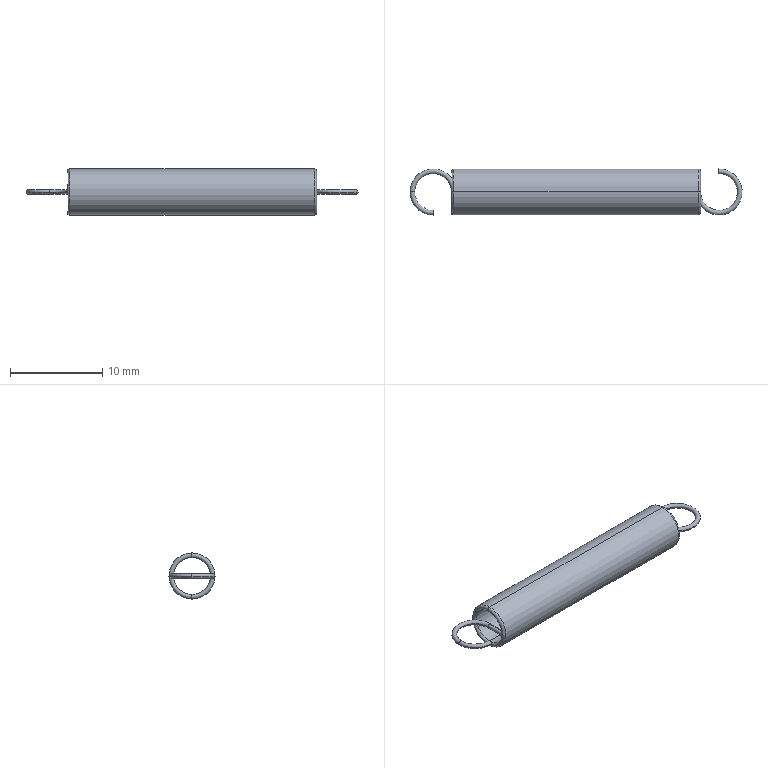Part | SolidWorks | features Revolution 5, RefAxis 2 | 1 solid | 20 faces | box 36 x 5 x 5 mm | volume 195.064 mm3 | torus 10 | cylinder 8 | plane 2 | commonest cylinder face diameters 0.5 x4 4 x2 5 x2
STEP:
#1=CARTESIAN_POINT('',(-0.5,0.,0.));
#2=VERTEX_POINT('',#1);
#3=CARTESIAN_POINT('',(0.,0.,0.));
#4=VERTEX_POINT('',#3);
#5=CARTESIAN_POINT('',(-0.25,0.,0.));
#6=DIRECTION('',(0.,-1.,0.));
#7=DIRECTION('',(0.,0.,-1.));
#8=AXIS2_PLACEMENT_3D('',#5,#6,#7);
#9=CIRCLE('',#8,0.25);
#10=EDGE_CURVE('',#2,#4,#9,.T.);
#11=ORIENTED_EDGE('',*,*,#10,.F.);
#12=CARTESIAN_POINT('',(4.5,0.,0.));
#13=VERTEX_POINT('',#12);
#14=CARTESIAN_POINT('',(2.,0.,0.));
#15=DIRECTION('',(0.,0.,-1.));
#16=DIRECTION('',(-1.,0.,0.));
#17=AXIS2_PLACEMENT_3D('',#14,#15,#16);
#18=CIRCLE('',#17,2.5);
#19=EDGE_CURVE('',#2,#13,#18,.T.);
#20=ORIENTED_EDGE('',*,*,#19,.T.);
#21=CARTESIAN_POINT('',(4.25,0.,-0.25));
#22=VERTEX_POINT('',#21);
#23=CARTESIAN_POINT('',(4.25,0.,0.));
#24=DIRECTION('',(0.,-1.,0.));
#25=DIRECTION('',(0.,0.,-1.));
#26=AXIS2_PLACEMENT_3D('',#23,#24,#25);
#27=CIRCLE('',#26,0.25);
#28=EDGE_CURVE('',#22,#13,#27,.T.);
#29=ORIENTED_EDGE('',*,*,#28,.F.);
#30=CARTESIAN_POINT('',(4.,0.,0.));
#31=VERTEX_POINT('',#30);
#32=CARTESIAN_POINT('',(4.25,0.,0.));
#33=DIRECTION('',(0.,-1.,0.));
#34=DIRECTION('',(0.,0.,-1.));
#35=AXIS2_PLACEMENT_3D('',#32,#33,#34);
#36=CIRCLE('',#35,0.25);
#37=EDGE_CURVE('',#31,#22,#36,.T.);
#38=ORIENTED_EDGE('',*,*,#37,.F.);
#39=CARTESIAN_POINT('',(2.,0.,0.));
#40=DIRECTION('',(0.,0.,-1.));
#41=DIRECTION('',(-1.,0.,0.));
#42=AXIS2_PLACEMENT_3D('',#39,#40,#41);
#43=CIRCLE('',#42,2.);
#44=EDGE_CURVE('',#4,#31,#43,.T.);
#45=ORIENTED_EDGE('',*,*,#44,.F.);
#46=EDGE_LOOP('',(#11,#20,#29,#38,#45));
#47=FACE_OUTER_BOUND('',#46,.T.);
#48=CARTESIAN_POINT('',(2.,0.,0.));
#49=DIRECTION('',(0.,0.,-1.));
#50=DIRECTION('',(-1.,0.,0.));
#51=AXIS2_PLACEMENT_3D('',#48,#49,#50);
#52=TOROIDAL_SURFACE('',#51,2.25,0.25);
#53=ADVANCED_FACE('',(#47),#52,.T.);
#54=CARTESIAN_POINT('',(32.965,2.,0.));
#55=VERTEX_POINT('',#54);
#56=CARTESIAN_POINT('',(32.956,2.5,0.));
#57=VERTEX_POINT('',#56);
#58=CARTESIAN_POINT('',(32.961,2.25,0.));
#59=DIRECTION('',(0.9998,0.01745,0.));
#60=DIRECTION('',(0.,0.,1.));
#61=AXIS2_PLACEMENT_3D('',#58,#59,#60);
#62=CIRCLE('',#61,0.25);
#63=EDGE_CURVE('',#55,#57,#62,.T.);
#64=ORIENTED_EDGE('',*,*,#63,.T.);
#65=CARTESIAN_POINT('',(30.5,0.,0.));
#66=VERTEX_POINT('',#65);
#67=CARTESIAN_POINT('',(33.,0.,0.));
#68=DIRECTION('',(0.,0.,-1.));
#69=DIRECTION('',(-1.,0.,0.));
#70=AXIS2_PLACEMENT_3D('',#67,#68,#69);
#71=CIRCLE('',#70,2.5);
#72=EDGE_CURVE('',#57,#66,#71,.T.);
#73=ORIENTED_EDGE('',*,*,#72,.T.);
#74=CARTESIAN_POINT('',(30.75,0.,-0.25));
#75=VERTEX_POINT('',#74);
#76=CARTESIAN_POINT('',(30.75,0.,0.));
#77=DIRECTION('',(0.,1.,0.));
#78=DIRECTION('',(0.,0.,1.));
#79=AXIS2_PLACEMENT_3D('',#76,#77,#78);
#80=CIRCLE('',#79,0.25);
#81=EDGE_CURVE('',#75,#66,#80,.T.);
#82=ORIENTED_EDGE('',*,*,#81,.F.);
#83=CARTESIAN_POINT('',(31.,0.,0.));
#84=VERTEX_POINT('',#83);
#85=CARTESIAN_POINT('',(30.75,0.,0.));
#86=DIRECTION('',(0.,1.,0.));
#87=DIRECTION('',(0.,0.,1.));
#88=AXIS2_PLACEMENT_3D('',#85,#86,#87);
#89=CIRCLE('',#88,0.25);
#90=EDGE_CURVE('',#84,#75,#89,.T.);
#91=ORIENTED_EDGE('',*,*,#90,.F.);
#92=CARTESIAN_POINT('',(33.,0.,0.));
#93=DIRECTION('',(0.,0.,-1.));
#94=DIRECTION('',(-1.,0.,0.));
#95=AXIS2_PLACEMENT_3D('',#92,#93,#94);
#96=CIRCLE('',#95,2.);
#97=EDGE_CURVE('',#55,#84,#96,.T.);
#98=ORIENTED_EDGE('',*,*,#97,.F.);
#99=EDGE_LOOP('',(#64,#73,#82,#91,#98));
#100=FACE_OUTER_BOUND('',#99,.T.);
#101=CARTESIAN_POINT('',(33.,0.,0.));
#102=DIRECTION('',(0.,0.,-1.));
#103=DIRECTION('',(-1.,0.,0.));
#104=AXIS2_PLACEMENT_3D('',#101,#102,#103);
#105=TOROIDAL_SURFACE('',#104,2.25,0.25);
#106=ADVANCED_FACE('',(#100),#105,.T.);
#107=CARTESIAN_POINT('',(2.044,-2.5,0.));
#108=VERTEX_POINT('',#107);
#109=CARTESIAN_POINT('',(2.035,-2.,0.));
#110=VERTEX_POINT('',#109);
#111=CARTESIAN_POINT('',(2.039,-2.25,0.));
#112=DIRECTION('',(0.9998,0.01745,0.));
#113=DIRECTION('',(0.,0.,1.));
#114=AXIS2_PLACEMENT_3D('',#111,#112,#113);
#115=CIRCLE('',#114,0.25);
#116=EDGE_CURVE('',#108,#110,#115,.T.);
#117=ORIENTED_EDGE('',*,*,#116,.F.);
#118=CARTESIAN_POINT('',(2.,0.,0.));
#119=DIRECTION('',(0.,0.,-1.));
#120=DIRECTION('',(-1.,0.,0.));
#121=AXIS2_PLACEMENT_3D('',#118,#119,#120);
#122=CIRCLE('',#121,2.5);
#123=EDGE_CURVE('',#108,#2,#122,.T.);
#124=ORIENTED_EDGE('',*,*,#123,.T.);
#125=ORIENTED_EDGE('',*,*,#10,.T.);
#126=CARTESIAN_POINT('',(2.,0.,0.));
#127=DIRECTION('',(0.,0.,-1.));
#128=DIRECTION('',(-1.,0.,0.));
#129=AXIS2_PLACEMENT_3D('',#126,#127,#128);
#130=CIRCLE('',#129,2.);
#131=EDGE_CURVE('',#110,#4,#130,.T.);
#132=ORIENTED_EDGE('',*,*,#131,.F.);
#133=EDGE_LOOP('',(#117,#124,#125,#132));
#134=FACE_OUTER_BOUND('',#133,.T.);
#135=CARTESIAN_POINT('',(2.,0.,0.));
#136=DIRECTION('',(0.,0.,-1.));
#137=DIRECTION('',(-1.,0.,0.));
#138=AXIS2_PLACEMENT_3D('',#135,#136,#137);
#139=TOROIDAL_SURFACE('',#138,2.25,0.25);
#140=ADVANCED_FACE('',(#134),#139,.T.);
#141=ORIENTED_EDGE('',*,*,#123,.F.);
#142=CARTESIAN_POINT('',(2.039,-2.25,0.));
#143=DIRECTION('',(0.9998,0.01745,0.));
#144=DIRECTION('',(0.,0.,1.));
#145=AXIS2_PLACEMENT_3D('',#142,#143,#144);
#146=CIRCLE('',#145,0.25);
#147=EDGE_CURVE('',#110,#108,#146,.T.);
#148=ORIENTED_EDGE('',*,*,#147,.F.);
#149=ORIENTED_EDGE('',*,*,#131,.T.);
#150=CARTESIAN_POINT('',(-0.25,0.,0.));
#151=DIRECTION('',(0.,-1.,0.));
#152=DIRECTION('',(0.,0.,-1.));
#153=AXIS2_PLACEMENT_3D('',#150,#151,#152);
#154=CIRCLE('',#153,0.25);
#155=EDGE_CURVE('',#4,#2,#154,.T.);
#156=ORIENTED_EDGE('',*,*,#155,.T.);
#157=EDGE_LOOP('',(#141,#148,#149,#156));
#158=FACE_OUTER_BOUND('',#157,.T.);
#159=CARTESIAN_POINT('',(2.,0.,0.));
#160=DIRECTION('',(0.,0.,-1.));
#161=DIRECTION('',(-1.,0.,0.));
#162=AXIS2_PLACEMENT_3D('',#159,#160,#161);
#163=TOROIDAL_SURFACE('',#162,2.25,0.25);
#164=ADVANCED_FACE('',(#158),#163,.T.);
#165=ORIENTED_EDGE('',*,*,#28,.T.);
#166=CARTESIAN_POINT('',(4.25,0.,0.25));
#167=VERTEX_POINT('',#166);
#168=CARTESIAN_POINT('',(4.25,0.,0.));
#169=DIRECTION('',(0.,-1.,0.));
#170=DIRECTION('',(0.,0.,-1.));
#171=AXIS2_PLACEMENT_3D('',#168,#169,#170);
#172=CIRCLE('',#171,0.25);
#173=EDGE_CURVE('',#13,#167,#172,.T.);
#174=ORIENTED_EDGE('',*,*,#173,.T.);
#175=CARTESIAN_POINT('',(4.25,-1.984,0.25));
#176=VERTEX_POINT('',#175);
#177=CARTESIAN_POINT('',(4.25,-2.25,0.25));
#178=DIRECTION('',(0.,-1.,0.));
#179=VECTOR('',#178,1000.);
#180=LINE('',#177,#179);
#181=EDGE_CURVE('',#167,#176,#180,.T.);
#182=ORIENTED_EDGE('',*,*,#181,.T.);
#183=CARTESIAN_POINT('',(4.25,-1.984,-0.25));
#184=VERTEX_POINT('',#183);
#185=CARTESIAN_POINT('',(4.25,-1.984,-0.25));
#186=CARTESIAN_POINT('',(4.316,-1.984,-0.25));
#187=CARTESIAN_POINT('',(4.381,-1.988,-0.2228));
#188=CARTESIAN_POINT('',(4.473,-1.996,-0.1307));
#189=CARTESIAN_POINT('',(4.5,-2.,-0.06539));
#190=CARTESIAN_POINT('',(4.5,-2.,0.0652));
#191=CARTESIAN_POINT('',(4.473,-1.996,0.1301));
#192=CARTESIAN_POINT('',(4.38,-1.988,0.2234));
#193=CARTESIAN_POINT('',(4.315,-1.984,0.25));
#194=CARTESIAN_POINT('',(4.25,-1.984,0.25));
#195=B_SPLINE_CURVE_WITH_KNOTS('',3,(#185,#186,#187,#188,#189,#190,#191,#192,#193,#194),.UNSPECIFIED.,.F.,.F.,(4,2,2,2,4),(0.,0.0001956,0.0003912,0.0005868,0.0007824),.UNSPECIFIED.);
#196=EDGE_CURVE('',#184,#176,#195,.T.);
#197=ORIENTED_EDGE('',*,*,#196,.F.);
#198=CARTESIAN_POINT('',(4.25,-2.25,-0.25));
#199=DIRECTION('',(0.,-1.,0.));
#200=VECTOR('',#199,1000.);
#201=LINE('',#198,#200);
#202=EDGE_CURVE('',#22,#184,#201,.T.);
#203=ORIENTED_EDGE('',*,*,#202,.F.);
#204=EDGE_LOOP('',(#165,#174,#182,#197,#203));
#205=FACE_OUTER_BOUND('',#204,.T.);
#206=CARTESIAN_POINT('',(4.25,-2.25,0.));
#207=DIRECTION('',(0.,-1.,0.));
#208=DIRECTION('',(0.,0.,-1.));
#209=AXIS2_PLACEMENT_3D('',#206,#207,#208);
#210=CYLINDRICAL_SURFACE('',#209,0.25);
#211=ADVANCED_FACE('',(#205),#210,.T.);
#212=CARTESIAN_POINT('',(30.75,0.,0.25));
#213=VERTEX_POINT('',#212);
#214=CARTESIAN_POINT('',(30.75,0.,0.));
#215=DIRECTION('',(0.,1.,0.));
#216=DIRECTION('',(0.,0.,1.));
#217=AXIS2_PLACEMENT_3D('',#214,#215,#216);
#218=CIRCLE('',#217,0.25);
#219=EDGE_CURVE('',#213,#84,#218,.T.);
#220=ORIENTED_EDGE('',*,*,#219,.T.);
#221=ORIENTED_EDGE('',*,*,#90,.T.);
#222=CARTESIAN_POINT('',(30.75,1.984,-0.25));
#223=VERTEX_POINT('',#222);
#224=CARTESIAN_POINT('',(30.75,0.,-0.25));
#225=DIRECTION('',(0.,1.,0.));
#226=VECTOR('',#225,1000.);
#227=LINE('',#224,#226);
#228=EDGE_CURVE('',#75,#223,#227,.T.);
#229=ORIENTED_EDGE('',*,*,#228,.T.);
#230=CARTESIAN_POINT('',(31.,2.25,0.));
#231=VERTEX_POINT('',#230);
#232=CARTESIAN_POINT('',(30.75,1.984,-0.25));
#233=CARTESIAN_POINT('',(30.791,1.984,-0.25));
#234=CARTESIAN_POINT('',(30.83,1.996,-0.2396));
#235=CARTESIAN_POINT('',(30.895,2.033,-0.2068));
#236=CARTESIAN_POINT('',(30.921,2.057,-0.1851));
#237=CARTESIAN_POINT('',(30.981,2.134,-0.1135));
#238=CARTESIAN_POINT('',(31.,2.193,-0.05703));
#239=CARTESIAN_POINT('',(31.,2.25,0.));
#240=B_SPLINE_CURVE_WITH_KNOTS('',3,(#232,#233,#234,#235,#236,#237,#238,#239),.UNSPECIFIED.,.F.,.F.,(4,2,2,4),(0.000000196,0.0001212,0.0002422,0.0004842),.UNSPECIFIED.);
#241=EDGE_CURVE('',#223,#231,#240,.T.);
#242=ORIENTED_EDGE('',*,*,#241,.T.);
#243=CARTESIAN_POINT('',(30.75,1.984,0.25));
#244=VERTEX_POINT('',#243);
#245=CARTESIAN_POINT('',(31.,2.25,0.));
#246=CARTESIAN_POINT('',(31.,2.193,0.05675));
#247=CARTESIAN_POINT('',(30.981,2.134,0.1135));
#248=CARTESIAN_POINT('',(30.921,2.057,0.1848));
#249=CARTESIAN_POINT('',(30.895,2.033,0.2066));
#250=CARTESIAN_POINT('',(30.831,1.996,0.2395));
#251=CARTESIAN_POINT('',(30.791,1.984,0.25));
#252=CARTESIAN_POINT('',(30.75,1.984,0.25));
#253=B_SPLINE_CURVE_WITH_KNOTS('',3,(#245,#246,#247,#248,#249,#250,#251,#252),.UNSPECIFIED.,.F.,.F.,(4,2,2,4),(-0.000003162,0.0002376,0.000358,0.0004785),.UNSPECIFIED.);
#254=EDGE_CURVE('',#231,#244,#253,.T.);
#255=ORIENTED_EDGE('',*,*,#254,.T.);
#256=CARTESIAN_POINT('',(30.75,0.,0.25));
#257=DIRECTION('',(0.,1.,0.));
#258=VECTOR('',#257,1000.);
#259=LINE('',#256,#258);
#260=EDGE_CURVE('',#213,#244,#259,.T.);
#261=ORIENTED_EDGE('',*,*,#260,.F.);
#262=EDGE_LOOP('',(#220,#221,#229,#242,#255,#261));
#263=FACE_OUTER_BOUND('',#262,.T.);
#264=CARTESIAN_POINT('',(30.75,0.,0.));
#265=DIRECTION('',(0.,1.,0.));
#266=DIRECTION('',(0.,0.,1.));
#267=AXIS2_PLACEMENT_3D('',#264,#265,#266);
#268=CYLINDRICAL_SURFACE('',#267,0.25);
#269=ADVANCED_FACE('',(#263),#268,.T.);
#270=CARTESIAN_POINT('',(30.75,0.,2.5));
#271=VERTEX_POINT('',#270);
#272=CARTESIAN_POINT('',(30.75,0.,-2.5));
#273=VERTEX_POINT('',#272);
#274=CARTESIAN_POINT('',(30.75,0.,0.));
#275=DIRECTION('',(-1.,0.,0.));
#276=DIRECTION('',(0.,0.,1.));
#277=AXIS2_PLACEMENT_3D('',#274,#275,#276);
#278=CIRCLE('',#277,2.5);
#279=EDGE_CURVE('',#271,#273,#278,.T.);
#280=ORIENTED_EDGE('',*,*,#279,.T.);
#281=CARTESIAN_POINT('',(4.25,0.,-2.5));
#282=VERTEX_POINT('',#281);
#283=CARTESIAN_POINT('',(31.,0.,-2.5));
#284=DIRECTION('',(-1.,0.,0.));
#285=VECTOR('',#284,1000.);
#286=LINE('',#283,#285);
#287=EDGE_CURVE('',#273,#282,#286,.T.);
#288=ORIENTED_EDGE('',*,*,#287,.T.);
#289=CARTESIAN_POINT('',(4.25,0.,2.5));
#290=VERTEX_POINT('',#289);
#291=CARTESIAN_POINT('',(4.25,0.,0.));
#292=DIRECTION('',(-1.,0.,0.));
#293=DIRECTION('',(0.,0.,1.));
#294=AXIS2_PLACEMENT_3D('',#291,#292,#293);
#295=CIRCLE('',#294,2.5);
#296=EDGE_CURVE('',#290,#282,#295,.T.);
#297=ORIENTED_EDGE('',*,*,#296,.F.);
#298=CARTESIAN_POINT('',(31.,0.,2.5));
#299=DIRECTION('',(-1.,0.,0.));
#300=VECTOR('',#299,1000.);
#301=LINE('',#298,#300);
#302=EDGE_CURVE('',#271,#290,#301,.T.);
#303=ORIENTED_EDGE('',*,*,#302,.F.);
#304=EDGE_LOOP('',(#280,#288,#297,#303));
#305=FACE_OUTER_BOUND('',#304,.T.);
#306=CARTESIAN_POINT('',(31.,0.,0.));
#307=DIRECTION('',(-1.,0.,0.));
#308=DIRECTION('',(0.,0.,1.));
#309=AXIS2_PLACEMENT_3D('',#306,#307,#308);
#310=CYLINDRICAL_SURFACE('',#309,2.5);
#311=ADVANCED_FACE('',(#305),#310,.T.);
#312=ORIENTED_EDGE('',*,*,#296,.T.);
#313=CARTESIAN_POINT('',(4.25,0.,-2.));
#314=VERTEX_POINT('',#313);
#315=CARTESIAN_POINT('',(4.25,0.,-2.25));
#316=DIRECTION('',(0.,1.,0.));
#317=DIRECTION('',(0.,0.,1.));
#318=AXIS2_PLACEMENT_3D('',#315,#316,#317);
#319=CIRCLE('',#318,0.25);
#320=EDGE_CURVE('',#282,#314,#319,.T.);
#321=ORIENTED_EDGE('',*,*,#320,.T.);
#322=CARTESIAN_POINT('',(4.25,0.,2.));
#323=VERTEX_POINT('',#322);
#324=CARTESIAN_POINT('',(4.25,0.,0.));
#325=DIRECTION('',(-1.,0.,0.));
#326=DIRECTION('',(0.,0.,1.));
#327=AXIS2_PLACEMENT_3D('',#324,#325,#326);
#328=CIRCLE('',#327,2.);
#329=EDGE_CURVE('',#323,#314,#328,.T.);
#330=ORIENTED_EDGE('',*,*,#329,.F.);
#331=CARTESIAN_POINT('',(4.25,0.,2.25));
#332=DIRECTION('',(0.,-1.,0.));
#333=DIRECTION('',(0.,0.,-1.));
#334=AXIS2_PLACEMENT_3D('',#331,#332,#333);
#335=CIRCLE('',#334,0.25);
#336=EDGE_CURVE('',#290,#323,#335,.T.);
#337=ORIENTED_EDGE('',*,*,#336,.F.);
#338=EDGE_LOOP('',(#312,#321,#330,#337));
#339=FACE_OUTER_BOUND('',#338,.T.);
#340=CARTESIAN_POINT('',(4.25,0.,0.));
#341=DIRECTION('',(-1.,0.,0.));
#342=DIRECTION('',(0.,0.,1.));
#343=AXIS2_PLACEMENT_3D('',#340,#341,#342);
#344=TOROIDAL_SURFACE('',#343,2.25,0.25);
#345=ADVANCED_FACE('',(#339),#344,.T.);
#346=CARTESIAN_POINT('',(30.75,0.,-2.));
#347=VERTEX_POINT('',#346);
#348=CARTESIAN_POINT('',(30.75,0.,0.));
#349=DIRECTION('',(-1.,0.,0.));
#350=DIRECTION('',(0.,0.,1.));
#351=AXIS2_PLACEMENT_3D('',#348,#349,#350);
#352=CIRCLE('',#351,2.);
#353=EDGE_CURVE('',#223,#347,#352,.T.);
#354=ORIENTED_EDGE('',*,*,#353,.T.);
#355=CARTESIAN_POINT('',(30.75,0.,-2.25));
#356=DIRECTION('',(0.,1.,0.));
#357=DIRECTION('',(0.,0.,1.));
#358=AXIS2_PLACEMENT_3D('',#355,#356,#357);
#359=CIRCLE('',#358,0.25);
#360=EDGE_CURVE('',#347,#273,#359,.T.);
#361=ORIENTED_EDGE('',*,*,#360,.T.);
#362=ORIENTED_EDGE('',*,*,#279,.F.);
#363=CARTESIAN_POINT('',(30.75,0.,2.));
#364=VERTEX_POINT('',#363);
#365=CARTESIAN_POINT('',(30.75,0.,2.25));
#366=DIRECTION('',(0.,-1.,0.));
#367=DIRECTION('',(0.,0.,-1.));
#368=AXIS2_PLACEMENT_3D('',#365,#366,#367);
#369=CIRCLE('',#368,0.25);
#370=EDGE_CURVE('',#364,#271,#369,.T.);
#371=ORIENTED_EDGE('',*,*,#370,.F.);
#372=CARTESIAN_POINT('',(30.75,0.,0.));
#373=DIRECTION('',(-1.,0.,0.));
#374=DIRECTION('',(0.,0.,1.));
#375=AXIS2_PLACEMENT_3D('',#372,#373,#374);
#376=CIRCLE('',#375,2.);
#377=EDGE_CURVE('',#364,#244,#376,.T.);
#378=ORIENTED_EDGE('',*,*,#377,.T.);
#379=ORIENTED_EDGE('',*,*,#254,.F.);
#380=ORIENTED_EDGE('',*,*,#241,.F.);
#381=EDGE_LOOP('',(#354,#361,#362,#371,#378,#379,#380));
#382=FACE_OUTER_BOUND('',#381,.T.);
#383=CARTESIAN_POINT('',(30.75,0.,0.));
#384=DIRECTION('',(-1.,0.,0.));
#385=DIRECTION('',(0.,0.,1.));
#386=AXIS2_PLACEMENT_3D('',#383,#384,#385);
#387=TOROIDAL_SURFACE('',#386,2.25,0.25);
#388=ADVANCED_FACE('',(#382),#387,.T.);
#389=CARTESIAN_POINT('',(30.75,0.,0.));
#390=DIRECTION('',(-1.,0.,0.));
#391=DIRECTION('',(0.,0.,1.));
#392=AXIS2_PLACEMENT_3D('',#389,#390,#391);
#393=CIRCLE('',#392,2.);
#394=EDGE_CURVE('',#347,#364,#393,.T.);
#395=ORIENTED_EDGE('',*,*,#394,.F.);
#396=CARTESIAN_POINT('',(31.,0.,-2.));
#397=DIRECTION('',(-1.,0.,0.));
#398=VECTOR('',#397,1000.);
#399=LINE('',#396,#398);
#400=EDGE_CURVE('',#347,#314,#399,.T.);
#401=ORIENTED_EDGE('',*,*,#400,.T.);
#402=CARTESIAN_POINT('',(4.25,0.,0.));
#403=DIRECTION('',(-1.,0.,0.));
#404=DIRECTION('',(0.,0.,1.));
#405=AXIS2_PLACEMENT_3D('',#402,#403,#404);
#406=CIRCLE('',#405,2.);
#407=EDGE_CURVE('',#314,#184,#406,.T.);
#408=ORIENTED_EDGE('',*,*,#407,.T.);
#409=ORIENTED_EDGE('',*,*,#196,.T.);
#410=CARTESIAN_POINT('',(4.25,0.,0.));
#411=DIRECTION('',(-1.,0.,0.));
#412=DIRECTION('',(0.,0.,1.));
#413=AXIS2_PLACEMENT_3D('',#410,#411,#412);
#414=CIRCLE('',#413,2.);
#415=EDGE_CURVE('',#176,#323,#414,.T.);
#416=ORIENTED_EDGE('',*,*,#415,.T.);
#417=CARTESIAN_POINT('',(31.,0.,2.));
#418=DIRECTION('',(-1.,0.,0.));
#419=VECTOR('',#418,1000.);
#420=LINE('',#417,#419);
#421=EDGE_CURVE('',#364,#323,#420,.T.);
#422=ORIENTED_EDGE('',*,*,#421,.F.);
#423=EDGE_LOOP('',(#395,#401,#408,#409,#416,#422));
#424=FACE_OUTER_BOUND('',#423,.T.);
#425=CARTESIAN_POINT('',(31.,0.,0.));
#426=DIRECTION('',(-1.,0.,0.));
#427=DIRECTION('',(0.,0.,1.));
#428=AXIS2_PLACEMENT_3D('',#425,#426,#427);
#429=CYLINDRICAL_SURFACE('',#428,2.);
#430=ADVANCED_FACE('',(#424),#429,.F.);
#431=ORIENTED_EDGE('',*,*,#400,.F.);
#432=ORIENTED_EDGE('',*,*,#353,.F.);
#433=CARTESIAN_POINT('',(30.75,1.984,0.25));
#434=CARTESIAN_POINT('',(30.684,1.984,0.25));
#435=CARTESIAN_POINT('',(30.619,1.988,0.2228));
#436=CARTESIAN_POINT('',(30.527,1.996,0.1307));
#437=CARTESIAN_POINT('',(30.5,2.,0.06539));
#438=CARTESIAN_POINT('',(30.5,2.,-0.0652));
#439=CARTESIAN_POINT('',(30.527,1.996,-0.1301));
#440=CARTESIAN_POINT('',(30.62,1.988,-0.2234));
#441=CARTESIAN_POINT('',(30.685,1.984,-0.25));
#442=CARTESIAN_POINT('',(30.75,1.984,-0.25));
#443=B_SPLINE_CURVE_WITH_KNOTS('',3,(#433,#434,#435,#436,#437,#438,#439,#440,#441,#442),.UNSPECIFIED.,.F.,.F.,(4,2,2,2,4),(0.,0.0001956,0.0003912,0.0005868,0.0007824),.UNSPECIFIED.);
#444=EDGE_CURVE('',#244,#223,#443,.T.);
#445=ORIENTED_EDGE('',*,*,#444,.F.);
#446=ORIENTED_EDGE('',*,*,#377,.F.);
#447=ORIENTED_EDGE('',*,*,#421,.T.);
#448=ORIENTED_EDGE('',*,*,#329,.T.);
#449=EDGE_LOOP('',(#431,#432,#445,#446,#447,#448));
#450=FACE_OUTER_BOUND('',#449,.T.);
#451=CARTESIAN_POINT('',(31.,0.,0.));
#452=DIRECTION('',(-1.,0.,0.));
#453=DIRECTION('',(0.,0.,1.));
#454=AXIS2_PLACEMENT_3D('',#451,#452,#453);
#455=CYLINDRICAL_SURFACE('',#454,2.);
#456=ADVANCED_FACE('',(#450),#455,.F.);
#457=ORIENTED_EDGE('',*,*,#360,.F.);
#458=ORIENTED_EDGE('',*,*,#394,.T.);
#459=ORIENTED_EDGE('',*,*,#370,.T.);
#460=CARTESIAN_POINT('',(30.75,0.,0.));
#461=DIRECTION('',(-1.,0.,0.));
#462=DIRECTION('',(0.,0.,1.));
#463=AXIS2_PLACEMENT_3D('',#460,#461,#462);
#464=CIRCLE('',#463,2.5);
#465=EDGE_CURVE('',#273,#271,#464,.T.);
#466=ORIENTED_EDGE('',*,*,#465,.F.);
#467=EDGE_LOOP('',(#457,#458,#459,#466));
#468=FACE_OUTER_BOUND('',#467,.T.);
#469=CARTESIAN_POINT('',(30.75,0.,0.));
#470=DIRECTION('',(-1.,0.,0.));
#471=DIRECTION('',(0.,0.,1.));
#472=AXIS2_PLACEMENT_3D('',#469,#470,#471);
#473=TOROIDAL_SURFACE('',#472,2.25,0.25);
#474=ADVANCED_FACE('',(#468),#473,.T.);
#475=ORIENTED_EDGE('',*,*,#320,.F.);
#476=CARTESIAN_POINT('',(4.25,0.,0.));
#477=DIRECTION('',(-1.,0.,0.));
#478=DIRECTION('',(0.,0.,1.));
#479=AXIS2_PLACEMENT_3D('',#476,#477,#478);
#480=CIRCLE('',#479,2.5);
#481=EDGE_CURVE('',#282,#290,#480,.T.);
#482=ORIENTED_EDGE('',*,*,#481,.T.);
#483=ORIENTED_EDGE('',*,*,#336,.T.);
#484=ORIENTED_EDGE('',*,*,#415,.F.);
#485=CARTESIAN_POINT('',(4.,-2.25,0.));
#486=VERTEX_POINT('',#485);
#487=CARTESIAN_POINT('',(4.25,-1.984,0.25));
#488=CARTESIAN_POINT('',(4.209,-1.984,0.25));
#489=CARTESIAN_POINT('',(4.17,-1.996,0.2396));
#490=CARTESIAN_POINT('',(4.105,-2.033,0.2068));
#491=CARTESIAN_POINT('',(4.079,-2.057,0.1851));
#492=CARTESIAN_POINT('',(4.019,-2.134,0.1135));
#493=CARTESIAN_POINT('',(4.,-2.193,0.05703));
#494=CARTESIAN_POINT('',(4.,-2.25,0.));
#495=B_SPLINE_CURVE_WITH_KNOTS('',3,(#487,#488,#489,#490,#491,#492,#493,#494),.UNSPECIFIED.,.F.,.F.,(4,2,2,4),(0.000000196,0.0001212,0.0002422,0.0004842),.UNSPECIFIED.);
#496=EDGE_CURVE('',#176,#486,#495,.T.);
#497=ORIENTED_EDGE('',*,*,#496,.T.);
#498=CARTESIAN_POINT('',(4.,-2.25,0.));
#499=CARTESIAN_POINT('',(4.,-2.193,-0.05675));
#500=CARTESIAN_POINT('',(4.019,-2.134,-0.1135));
#501=CARTESIAN_POINT('',(4.079,-2.057,-0.1848));
#502=CARTESIAN_POINT('',(4.105,-2.033,-0.2066));
#503=CARTESIAN_POINT('',(4.169,-1.996,-0.2395));
#504=CARTESIAN_POINT('',(4.209,-1.984,-0.25));
#505=CARTESIAN_POINT('',(4.25,-1.984,-0.25));
#506=B_SPLINE_CURVE_WITH_KNOTS('',3,(#498,#499,#500,#501,#502,#503,#504,#505),.UNSPECIFIED.,.F.,.F.,(4,2,2,4),(-0.000003162,0.0002376,0.000358,0.0004785),.UNSPECIFIED.);
#507=EDGE_CURVE('',#486,#184,#506,.T.);
#508=ORIENTED_EDGE('',*,*,#507,.T.);
#509=ORIENTED_EDGE('',*,*,#407,.F.);
#510=EDGE_LOOP('',(#475,#482,#483,#484,#497,#508,#509));
#511=FACE_OUTER_BOUND('',#510,.T.);
#512=CARTESIAN_POINT('',(4.25,0.,0.));
#513=DIRECTION('',(-1.,0.,0.));
#514=DIRECTION('',(0.,0.,1.));
#515=AXIS2_PLACEMENT_3D('',#512,#513,#514);
#516=TOROIDAL_SURFACE('',#515,2.25,0.25);
#517=ADVANCED_FACE('',(#511),#516,.T.);
#518=ORIENTED_EDGE('',*,*,#287,.F.);
#519=ORIENTED_EDGE('',*,*,#465,.T.);
#520=ORIENTED_EDGE('',*,*,#302,.T.);
#521=ORIENTED_EDGE('',*,*,#481,.F.);
#522=EDGE_LOOP('',(#518,#519,#520,#521));
#523=FACE_OUTER_BOUND('',#522,.T.);
#524=CARTESIAN_POINT('',(31.,0.,0.));
#525=DIRECTION('',(-1.,0.,0.));
#526=DIRECTION('',(0.,0.,1.));
#527=AXIS2_PLACEMENT_3D('',#524,#525,#526);
#528=CYLINDRICAL_SURFACE('',#527,2.5);
#529=ADVANCED_FACE('',(#523),#528,.T.);
#530=ORIENTED_EDGE('',*,*,#228,.F.);
#531=ORIENTED_EDGE('',*,*,#81,.T.);
#532=CARTESIAN_POINT('',(30.75,0.,0.));
#533=DIRECTION('',(0.,1.,0.));
#534=DIRECTION('',(0.,0.,1.));
#535=AXIS2_PLACEMENT_3D('',#532,#533,#534);
#536=CIRCLE('',#535,0.25);
#537=EDGE_CURVE('',#66,#213,#536,.T.);
#538=ORIENTED_EDGE('',*,*,#537,.T.);
#539=ORIENTED_EDGE('',*,*,#260,.T.);
#540=ORIENTED_EDGE('',*,*,#444,.T.);
#541=EDGE_LOOP('',(#530,#531,#538,#539,#540));
#542=FACE_OUTER_BOUND('',#541,.T.);
#543=CARTESIAN_POINT('',(30.75,0.,0.));
#544=DIRECTION('',(0.,1.,0.));
#545=DIRECTION('',(0.,0.,1.));
#546=AXIS2_PLACEMENT_3D('',#543,#544,#545);
#547=CYLINDRICAL_SURFACE('',#546,0.25);
#548=ADVANCED_FACE('',(#542),#547,.T.);
#549=ORIENTED_EDGE('',*,*,#72,.F.);
#550=CARTESIAN_POINT('',(32.961,2.25,0.));
#551=DIRECTION('',(0.9998,0.01745,0.));
#552=DIRECTION('',(0.,0.,1.));
#553=AXIS2_PLACEMENT_3D('',#550,#551,#552);
#554=CIRCLE('',#553,0.25);
#555=EDGE_CURVE('',#57,#55,#554,.T.);
#556=ORIENTED_EDGE('',*,*,#555,.T.);
#557=ORIENTED_EDGE('',*,*,#97,.T.);
#558=ORIENTED_EDGE('',*,*,#219,.F.);
#559=ORIENTED_EDGE('',*,*,#537,.F.);
#560=EDGE_LOOP('',(#549,#556,#557,#558,#559));
#561=FACE_OUTER_BOUND('',#560,.T.);
#562=CARTESIAN_POINT('',(33.,0.,0.));
#563=DIRECTION('',(0.,0.,-1.));
#564=DIRECTION('',(-1.,0.,0.));
#565=AXIS2_PLACEMENT_3D('',#562,#563,#564);
#566=TOROIDAL_SURFACE('',#565,2.25,0.25);
#567=ADVANCED_FACE('',(#561),#566,.T.);
#568=ORIENTED_EDGE('',*,*,#63,.F.);
#569=ORIENTED_EDGE('',*,*,#555,.F.);
#570=EDGE_LOOP('',(#568,#569));
#571=FACE_OUTER_BOUND('',#570,.T.);
#572=CARTESIAN_POINT('',(32.961,2.25,0.));
#573=DIRECTION('',(0.9998,0.01745,0.));
#574=DIRECTION('',(0.,0.,1.));
#575=AXIS2_PLACEMENT_3D('',#572,#573,#574);
#576=PLANE('',#575);
#577=ADVANCED_FACE('',(#571),#576,.F.);
#578=ORIENTED_EDGE('',*,*,#181,.F.);
#579=CARTESIAN_POINT('',(4.25,0.,0.));
#580=DIRECTION('',(0.,-1.,0.));
#581=DIRECTION('',(0.,0.,-1.));
#582=AXIS2_PLACEMENT_3D('',#579,#580,#581);
#583=CIRCLE('',#582,0.25);
#584=EDGE_CURVE('',#167,#31,#583,.T.);
#585=ORIENTED_EDGE('',*,*,#584,.T.);
#586=ORIENTED_EDGE('',*,*,#37,.T.);
#587=ORIENTED_EDGE('',*,*,#202,.T.);
#588=ORIENTED_EDGE('',*,*,#507,.F.);
#589=ORIENTED_EDGE('',*,*,#496,.F.);
#590=EDGE_LOOP('',(#578,#585,#586,#587,#588,#589));
#591=FACE_OUTER_BOUND('',#590,.T.);
#592=CARTESIAN_POINT('',(4.25,-2.25,0.));
#593=DIRECTION('',(0.,-1.,0.));
#594=DIRECTION('',(0.,0.,-1.));
#595=AXIS2_PLACEMENT_3D('',#592,#593,#594);
#596=CYLINDRICAL_SURFACE('',#595,0.25);
#597=ADVANCED_FACE('',(#591),#596,.T.);
#598=ORIENTED_EDGE('',*,*,#19,.F.);
#599=ORIENTED_EDGE('',*,*,#155,.F.);
#600=ORIENTED_EDGE('',*,*,#44,.T.);
#601=ORIENTED_EDGE('',*,*,#584,.F.);
#602=ORIENTED_EDGE('',*,*,#173,.F.);
#603=EDGE_LOOP('',(#598,#599,#600,#601,#602));
#604=FACE_OUTER_BOUND('',#603,.T.);
#605=CARTESIAN_POINT('',(2.,0.,0.));
#606=DIRECTION('',(0.,0.,-1.));
#607=DIRECTION('',(-1.,0.,0.));
#608=AXIS2_PLACEMENT_3D('',#605,#606,#607);
#609=TOROIDAL_SURFACE('',#608,2.25,0.25);
#610=ADVANCED_FACE('',(#604),#609,.T.);
#611=ORIENTED_EDGE('',*,*,#147,.T.);
#612=ORIENTED_EDGE('',*,*,#116,.T.);
#613=EDGE_LOOP('',(#611,#612));
#614=FACE_OUTER_BOUND('',#613,.T.);
#615=CARTESIAN_POINT('',(2.039,-2.25,0.));
#616=DIRECTION('',(0.9998,0.01745,0.));
#617=DIRECTION('',(0.,0.,1.));
#618=AXIS2_PLACEMENT_3D('',#615,#616,#617);
#619=PLANE('',#618);
#620=ADVANCED_FACE('',(#614),#619,.T.);
#621=CLOSED_SHELL('',(#53,#106,#140,#164,#211,#269,#311,#345,#388,#430,#456,#474,#517,#529,#548,#567,#577,#597,#610,#620));
#622=MANIFOLD_SOLID_BREP('',#621);
#623=CARTESIAN_POINT('',(0.,0.,0.));
#624=DIRECTION('',(0.,0.,1.));
#625=DIRECTION('',(1.,0.,0.));
#626=AXIS2_PLACEMENT_3D('',#623,#624,#625);
#627=(LENGTH_UNIT()NAMED_UNIT(*)SI_UNIT(.MILLI.,.METRE.));
#628=UNCERTAINTY_MEASURE_WITH_UNIT(LENGTH_MEASURE(0.00001),#627,'','');
#629=(NAMED_UNIT(*)PLANE_ANGLE_UNIT()SI_UNIT($,.RADIAN.));
#630=(NAMED_UNIT(*)SI_UNIT($,.STERADIAN.)SOLID_ANGLE_UNIT());
#631=(GEOMETRIC_REPRESENTATION_CONTEXT(3)GLOBAL_UNCERTAINTY_ASSIGNED_CONTEXT((#628))GLOBAL_UNIT_ASSIGNED_CONTEXT((#627,#629,#630))REPRESENTATION_CONTEXT('',''));
#632=ADVANCED_BREP_SHAPE_REPRESENTATION('',(#622,#626),#631);